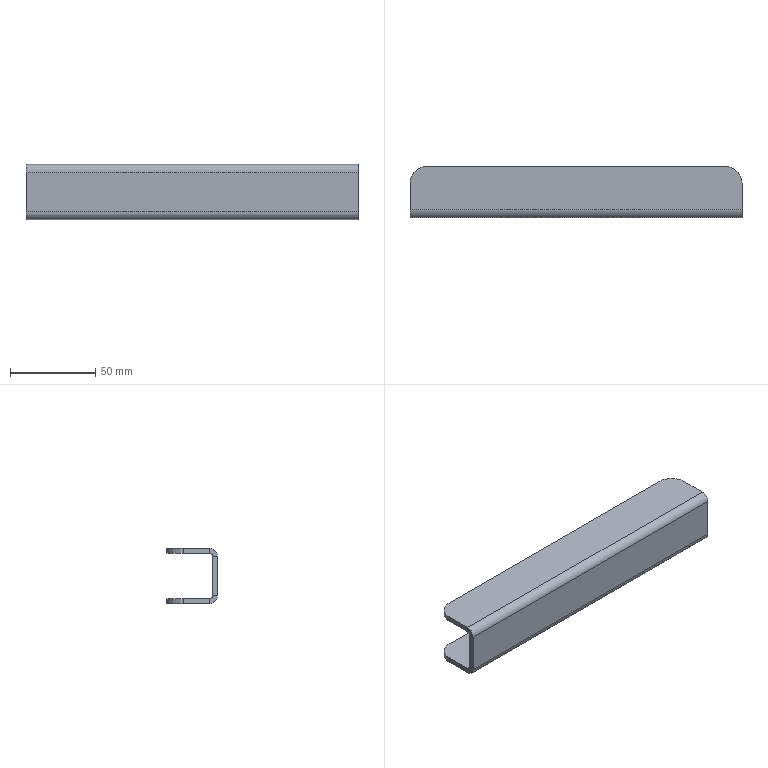Part | NX | features BREP 1 | 1 solid | 26 faces | box 195.072 x 29.972 x 32.487 mm | volume 48731 mm3 | plane 18 | cylinder 8 | commonest cylinder face diameters 19.964 x4 3.175 x2 9.169 x2
STEP:
#1=CARTESIAN_POINT('',(-97.536,0.,11.659));
#2=VERTEX_POINT('',#1);
#3=CARTESIAN_POINT('',(97.536,0.,11.659));
#4=VERTEX_POINT('',#3);
#5=CARTESIAN_POINT('',(-97.536,0.,11.659));
#6=DIRECTION('',(1.,0.,0.));
#7=VECTOR('',#6,1000.);
#8=LINE('',#5,#7);
#9=EDGE_CURVE('',#2,#4,#8,.T.);
#10=ORIENTED_EDGE('',*,*,#9,.T.);
#11=CARTESIAN_POINT('',(97.536,0.,-11.659));
#12=VERTEX_POINT('',#11);
#13=CARTESIAN_POINT('',(97.536,0.,11.659));
#14=DIRECTION('',(0.,0.,-1.));
#15=VECTOR('',#14,1000.);
#16=LINE('',#13,#15);
#17=EDGE_CURVE('',#4,#12,#16,.T.);
#18=ORIENTED_EDGE('',*,*,#17,.T.);
#19=CARTESIAN_POINT('',(-97.536,0.,-11.659));
#20=VERTEX_POINT('',#19);
#21=CARTESIAN_POINT('',(97.536,0.,-11.659));
#22=DIRECTION('',(-1.,0.,0.));
#23=VECTOR('',#22,1000.);
#24=LINE('',#21,#23);
#25=EDGE_CURVE('',#12,#20,#24,.T.);
#26=ORIENTED_EDGE('',*,*,#25,.T.);
#27=CARTESIAN_POINT('',(-97.536,0.,-11.659));
#28=DIRECTION('',(0.,0.,1.));
#29=VECTOR('',#28,1000.);
#30=LINE('',#27,#29);
#31=EDGE_CURVE('',#20,#2,#30,.T.);
#32=ORIENTED_EDGE('',*,*,#31,.T.);
#33=EDGE_LOOP('',(#10,#18,#26,#32));
#34=FACE_BOUND('',#33,.T.);
#35=CARTESIAN_POINT('',(0.,0.,0.));
#36=DIRECTION('',(0.,1.,0.));
#37=DIRECTION('',(1.,0.,0.));
#38=AXIS2_PLACEMENT_3D('',#35,#36,#37);
#39=PLANE('',#38);
#40=ADVANCED_FACE('',(#34),#39,.T.);
#41=CARTESIAN_POINT('',(-97.536,-2.997,-11.659));
#42=VERTEX_POINT('',#41);
#43=CARTESIAN_POINT('',(-97.536,0.,-11.659));
#44=DIRECTION('',(0.,-1.,0.));
#45=VECTOR('',#44,1000.);
#46=LINE('',#43,#45);
#47=EDGE_CURVE('',#20,#42,#46,.T.);
#48=ORIENTED_EDGE('',*,*,#47,.T.);
#49=CARTESIAN_POINT('',(-97.536,-2.997,11.659));
#50=VERTEX_POINT('',#49);
#51=CARTESIAN_POINT('',(-97.536,-2.997,-11.659));
#52=DIRECTION('',(0.,0.,1.));
#53=VECTOR('',#52,1000.);
#54=LINE('',#51,#53);
#55=EDGE_CURVE('',#42,#50,#54,.T.);
#56=ORIENTED_EDGE('',*,*,#55,.T.);
#57=CARTESIAN_POINT('',(-97.536,0.,11.659));
#58=DIRECTION('',(0.,-1.,0.));
#59=VECTOR('',#58,1000.);
#60=LINE('',#57,#59);
#61=EDGE_CURVE('',#2,#50,#60,.T.);
#62=ORIENTED_EDGE('',*,*,#61,.F.);
#63=ORIENTED_EDGE('',*,*,#31,.F.);
#64=EDGE_LOOP('',(#48,#56,#62,#63));
#65=FACE_BOUND('',#64,.T.);
#66=CARTESIAN_POINT('',(-97.536,-1.499,0.));
#67=DIRECTION('',(-1.,0.,0.));
#68=DIRECTION('',(0.,0.,1.));
#69=AXIS2_PLACEMENT_3D('',#66,#67,#68);
#70=PLANE('',#69);
#71=ADVANCED_FACE('',(#65),#70,.T.);
#72=ORIENTED_EDGE('',*,*,#61,.T.);
#73=CARTESIAN_POINT('',(-97.536,1.587,16.243));
#74=VERTEX_POINT('',#73);
#75=CARTESIAN_POINT('',(-97.536,1.587,11.659));
#76=DIRECTION('',(1.,0.,0.));
#77=DIRECTION('',(0.,0.,1.));
#78=AXIS2_PLACEMENT_3D('',#75,#76,#77);
#79=CIRCLE('',#78,4.585);
#80=EDGE_CURVE('',#74,#50,#79,.T.);
#81=ORIENTED_EDGE('',*,*,#80,.F.);
#82=CARTESIAN_POINT('',(-97.536,1.587,13.246));
#83=VERTEX_POINT('',#82);
#84=CARTESIAN_POINT('',(-97.536,1.587,13.246));
#85=DIRECTION('',(0.,0.,1.));
#86=VECTOR('',#85,1000.);
#87=LINE('',#84,#86);
#88=EDGE_CURVE('',#83,#74,#87,.T.);
#89=ORIENTED_EDGE('',*,*,#88,.F.);
#90=CARTESIAN_POINT('',(-97.536,1.587,11.659));
#91=DIRECTION('',(1.,0.,0.));
#92=DIRECTION('',(0.,0.,1.));
#93=AXIS2_PLACEMENT_3D('',#90,#91,#92);
#94=CIRCLE('',#93,1.587);
#95=EDGE_CURVE('',#83,#2,#94,.T.);
#96=ORIENTED_EDGE('',*,*,#95,.T.);
#97=EDGE_LOOP('',(#72,#81,#89,#96));
#98=FACE_BOUND('',#97,.T.);
#99=CARTESIAN_POINT('',(-97.536,-0.5947,13.841));
#100=DIRECTION('',(1.,0.,0.));
#101=DIRECTION('',(0.,1.,0.));
#102=AXIS2_PLACEMENT_3D('',#99,#100,#101);
#103=PLANE('',#102);
#104=ADVANCED_FACE('',(#98),#103,.F.);
#105=CARTESIAN_POINT('',(97.536,1.587,13.246));
#106=VERTEX_POINT('',#105);
#107=CARTESIAN_POINT('',(97.536,1.587,11.659));
#108=DIRECTION('',(1.,0.,0.));
#109=DIRECTION('',(0.,0.,1.));
#110=AXIS2_PLACEMENT_3D('',#107,#108,#109);
#111=CIRCLE('',#110,1.587);
#112=EDGE_CURVE('',#106,#4,#111,.T.);
#113=ORIENTED_EDGE('',*,*,#112,.T.);
#114=ORIENTED_EDGE('',*,*,#9,.F.);
#115=ORIENTED_EDGE('',*,*,#95,.F.);
#116=CARTESIAN_POINT('',(-97.536,1.587,13.246));
#117=DIRECTION('',(1.,0.,0.));
#118=VECTOR('',#117,1000.);
#119=LINE('',#116,#118);
#120=EDGE_CURVE('',#83,#106,#119,.T.);
#121=ORIENTED_EDGE('',*,*,#120,.T.);
#122=EDGE_LOOP('',(#113,#114,#115,#121));
#123=FACE_BOUND('',#122,.T.);
#124=CARTESIAN_POINT('',(-97.536,1.587,11.659));
#125=DIRECTION('',(1.,0.,0.));
#126=DIRECTION('',(0.,0.,1.));
#127=AXIS2_PLACEMENT_3D('',#124,#125,#126);
#128=CYLINDRICAL_SURFACE('',#127,1.587);
#129=ADVANCED_FACE('',(#123),#128,.F.);
#130=CARTESIAN_POINT('',(97.536,16.993,13.246));
#131=VERTEX_POINT('',#130);
#132=CARTESIAN_POINT('',(97.536,1.587,13.246));
#133=DIRECTION('',(0.,1.,0.));
#134=VECTOR('',#133,1000.);
#135=LINE('',#132,#134);
#136=EDGE_CURVE('',#106,#131,#135,.T.);
#137=ORIENTED_EDGE('',*,*,#136,.F.);
#138=ORIENTED_EDGE('',*,*,#120,.F.);
#139=CARTESIAN_POINT('',(-97.536,16.993,13.246));
#140=VERTEX_POINT('',#139);
#141=CARTESIAN_POINT('',(-97.536,16.993,13.246));
#142=DIRECTION('',(0.,-1.,0.));
#143=VECTOR('',#142,1000.);
#144=LINE('',#141,#143);
#145=EDGE_CURVE('',#140,#83,#144,.T.);
#146=ORIENTED_EDGE('',*,*,#145,.F.);
#147=CARTESIAN_POINT('',(-87.554,26.975,13.246));
#148=VERTEX_POINT('',#147);
#149=CARTESIAN_POINT('',(-87.554,16.993,13.246));
#150=DIRECTION('',(0.,0.,-1.));
#151=DIRECTION('',(-1.,0.,0.));
#152=AXIS2_PLACEMENT_3D('',#149,#150,#151);
#153=CIRCLE('',#152,9.982);
#154=EDGE_CURVE('',#140,#148,#153,.T.);
#155=ORIENTED_EDGE('',*,*,#154,.T.);
#156=CARTESIAN_POINT('',(87.554,26.975,13.246));
#157=VERTEX_POINT('',#156);
#158=CARTESIAN_POINT('',(87.554,26.975,13.246));
#159=DIRECTION('',(-1.,0.,0.));
#160=VECTOR('',#159,1000.);
#161=LINE('',#158,#160);
#162=EDGE_CURVE('',#157,#148,#161,.T.);
#163=ORIENTED_EDGE('',*,*,#162,.F.);
#164=CARTESIAN_POINT('',(87.554,16.993,13.246));
#165=DIRECTION('',(0.,0.,-1.));
#166=DIRECTION('',(0.,1.,0.));
#167=AXIS2_PLACEMENT_3D('',#164,#165,#166);
#168=CIRCLE('',#167,9.982);
#169=EDGE_CURVE('',#157,#131,#168,.T.);
#170=ORIENTED_EDGE('',*,*,#169,.T.);
#171=EDGE_LOOP('',(#137,#138,#146,#155,#163,#170));
#172=FACE_BOUND('',#171,.T.);
#173=CARTESIAN_POINT('',(-51.187,0.,13.246));
#174=DIRECTION('',(0.,0.,1.));
#175=DIRECTION('',(1.,0.,0.));
#176=AXIS2_PLACEMENT_3D('',#173,#174,#175);
#177=PLANE('',#176);
#178=ADVANCED_FACE('',(#172),#177,.F.);
#179=CARTESIAN_POINT('',(97.536,16.993,16.243));
#180=VERTEX_POINT('',#179);
#181=CARTESIAN_POINT('',(87.554,26.975,16.243));
#182=VERTEX_POINT('',#181);
#183=CARTESIAN_POINT('',(87.554,16.993,16.243));
#184=DIRECTION('',(0.,0.,1.));
#185=DIRECTION('',(1.,0.,0.));
#186=AXIS2_PLACEMENT_3D('',#183,#184,#185);
#187=CIRCLE('',#186,9.982);
#188=EDGE_CURVE('',#180,#182,#187,.T.);
#189=ORIENTED_EDGE('',*,*,#188,.F.);
#190=CARTESIAN_POINT('',(97.536,16.993,16.243));
#191=DIRECTION('',(0.,0.,-1.));
#192=VECTOR('',#191,1000.);
#193=LINE('',#190,#192);
#194=EDGE_CURVE('',#180,#131,#193,.T.);
#195=ORIENTED_EDGE('',*,*,#194,.T.);
#196=ORIENTED_EDGE('',*,*,#169,.F.);
#197=CARTESIAN_POINT('',(87.554,26.975,16.243));
#198=DIRECTION('',(0.,0.,-1.));
#199=VECTOR('',#198,1000.);
#200=LINE('',#197,#199);
#201=EDGE_CURVE('',#182,#157,#200,.T.);
#202=ORIENTED_EDGE('',*,*,#201,.F.);
#203=EDGE_LOOP('',(#189,#195,#196,#202));
#204=FACE_BOUND('',#203,.T.);
#205=CARTESIAN_POINT('',(87.554,16.993,16.533));
#206=DIRECTION('',(0.,0.,-1.));
#207=DIRECTION('',(0.,1.,0.));
#208=AXIS2_PLACEMENT_3D('',#205,#206,#207);
#209=CYLINDRICAL_SURFACE('',#208,9.982);
#210=ADVANCED_FACE('',(#204),#209,.T.);
#211=ORIENTED_EDGE('',*,*,#162,.T.);
#212=CARTESIAN_POINT('',(-87.554,26.975,16.243));
#213=VERTEX_POINT('',#212);
#214=CARTESIAN_POINT('',(-87.554,26.975,16.243));
#215=DIRECTION('',(0.,0.,-1.));
#216=VECTOR('',#215,1000.);
#217=LINE('',#214,#216);
#218=EDGE_CURVE('',#213,#148,#217,.T.);
#219=ORIENTED_EDGE('',*,*,#218,.F.);
#220=CARTESIAN_POINT('',(87.554,26.975,16.243));
#221=DIRECTION('',(-1.,0.,0.));
#222=VECTOR('',#221,1000.);
#223=LINE('',#220,#222);
#224=EDGE_CURVE('',#182,#213,#223,.T.);
#225=ORIENTED_EDGE('',*,*,#224,.F.);
#226=ORIENTED_EDGE('',*,*,#201,.T.);
#227=EDGE_LOOP('',(#211,#219,#225,#226));
#228=FACE_BOUND('',#227,.T.);
#229=CARTESIAN_POINT('',(0.,26.975,14.745));
#230=DIRECTION('',(0.,-1.,0.));
#231=DIRECTION('',(0.,0.,-1.));
#232=AXIS2_PLACEMENT_3D('',#229,#230,#231);
#233=PLANE('',#232);
#234=ADVANCED_FACE('',(#228),#233,.F.);
#235=ORIENTED_EDGE('',*,*,#224,.T.);
#236=CARTESIAN_POINT('',(-97.536,16.993,16.243));
#237=VERTEX_POINT('',#236);
#238=CARTESIAN_POINT('',(-87.554,16.993,16.243));
#239=DIRECTION('',(0.,0.,1.));
#240=DIRECTION('',(0.,1.,0.));
#241=AXIS2_PLACEMENT_3D('',#238,#239,#240);
#242=CIRCLE('',#241,9.982);
#243=EDGE_CURVE('',#213,#237,#242,.T.);
#244=ORIENTED_EDGE('',*,*,#243,.T.);
#245=CARTESIAN_POINT('',(-97.536,16.993,16.243));
#246=DIRECTION('',(0.,-1.,0.));
#247=VECTOR('',#246,1000.);
#248=LINE('',#245,#247);
#249=EDGE_CURVE('',#237,#74,#248,.T.);
#250=ORIENTED_EDGE('',*,*,#249,.T.);
#251=CARTESIAN_POINT('',(97.536,1.587,16.243));
#252=VERTEX_POINT('',#251);
#253=CARTESIAN_POINT('',(-97.536,1.587,16.243));
#254=DIRECTION('',(1.,0.,0.));
#255=VECTOR('',#254,1000.);
#256=LINE('',#253,#255);
#257=EDGE_CURVE('',#74,#252,#256,.T.);
#258=ORIENTED_EDGE('',*,*,#257,.T.);
#259=CARTESIAN_POINT('',(97.536,1.587,16.243));
#260=DIRECTION('',(0.,1.,0.));
#261=VECTOR('',#260,1000.);
#262=LINE('',#259,#261);
#263=EDGE_CURVE('',#252,#180,#262,.T.);
#264=ORIENTED_EDGE('',*,*,#263,.T.);
#265=ORIENTED_EDGE('',*,*,#188,.T.);
#266=EDGE_LOOP('',(#235,#244,#250,#258,#264,#265));
#267=FACE_BOUND('',#266,.T.);
#268=CARTESIAN_POINT('',(-51.187,0.,16.243));
#269=DIRECTION('',(0.,0.,1.));
#270=DIRECTION('',(1.,0.,0.));
#271=AXIS2_PLACEMENT_3D('',#268,#269,#270);
#272=PLANE('',#271);
#273=ADVANCED_FACE('',(#267),#272,.T.);
#274=ORIENTED_EDGE('',*,*,#263,.F.);
#275=CARTESIAN_POINT('',(97.536,1.587,13.246));
#276=DIRECTION('',(0.,0.,1.));
#277=VECTOR('',#276,1000.);
#278=LINE('',#275,#277);
#279=EDGE_CURVE('',#106,#252,#278,.T.);
#280=ORIENTED_EDGE('',*,*,#279,.F.);
#281=ORIENTED_EDGE('',*,*,#136,.T.);
#282=ORIENTED_EDGE('',*,*,#194,.F.);
#283=EDGE_LOOP('',(#274,#280,#281,#282));
#284=FACE_BOUND('',#283,.T.);
#285=CARTESIAN_POINT('',(97.536,14.281,14.745));
#286=DIRECTION('',(-1.,0.,0.));
#287=DIRECTION('',(0.,0.,1.));
#288=AXIS2_PLACEMENT_3D('',#285,#286,#287);
#289=PLANE('',#288);
#290=ADVANCED_FACE('',(#284),#289,.F.);
#291=ORIENTED_EDGE('',*,*,#279,.T.);
#292=CARTESIAN_POINT('',(97.536,-2.997,11.659));
#293=VERTEX_POINT('',#292);
#294=CARTESIAN_POINT('',(97.536,1.587,11.659));
#295=DIRECTION('',(1.,0.,0.));
#296=DIRECTION('',(0.,0.,1.));
#297=AXIS2_PLACEMENT_3D('',#294,#295,#296);
#298=CIRCLE('',#297,4.585);
#299=EDGE_CURVE('',#252,#293,#298,.T.);
#300=ORIENTED_EDGE('',*,*,#299,.T.);
#301=CARTESIAN_POINT('',(97.536,0.,11.659));
#302=DIRECTION('',(0.,-1.,0.));
#303=VECTOR('',#302,1000.);
#304=LINE('',#301,#303);
#305=EDGE_CURVE('',#4,#293,#304,.T.);
#306=ORIENTED_EDGE('',*,*,#305,.F.);
#307=ORIENTED_EDGE('',*,*,#112,.F.);
#308=EDGE_LOOP('',(#291,#300,#306,#307));
#309=FACE_BOUND('',#308,.T.);
#310=CARTESIAN_POINT('',(97.536,-0.5947,13.841));
#311=DIRECTION('',(1.,0.,0.));
#312=DIRECTION('',(0.,1.,0.));
#313=AXIS2_PLACEMENT_3D('',#310,#311,#312);
#314=PLANE('',#313);
#315=ADVANCED_FACE('',(#309),#314,.T.);
#316=ORIENTED_EDGE('',*,*,#305,.T.);
#317=CARTESIAN_POINT('',(97.536,-2.997,-11.659));
#318=VERTEX_POINT('',#317);
#319=CARTESIAN_POINT('',(97.536,-2.997,11.659));
#320=DIRECTION('',(0.,0.,-1.));
#321=VECTOR('',#320,1000.);
#322=LINE('',#319,#321);
#323=EDGE_CURVE('',#293,#318,#322,.T.);
#324=ORIENTED_EDGE('',*,*,#323,.T.);
#325=CARTESIAN_POINT('',(97.536,0.,-11.659));
#326=DIRECTION('',(0.,-1.,0.));
#327=VECTOR('',#326,1000.);
#328=LINE('',#325,#327);
#329=EDGE_CURVE('',#12,#318,#328,.T.);
#330=ORIENTED_EDGE('',*,*,#329,.F.);
#331=ORIENTED_EDGE('',*,*,#17,.F.);
#332=EDGE_LOOP('',(#316,#324,#330,#331));
#333=FACE_BOUND('',#332,.T.);
#334=CARTESIAN_POINT('',(97.536,-1.499,0.));
#335=DIRECTION('',(1.,0.,0.));
#336=DIRECTION('',(0.,1.,0.));
#337=AXIS2_PLACEMENT_3D('',#334,#335,#336);
#338=PLANE('',#337);
#339=ADVANCED_FACE('',(#333),#338,.T.);
#340=ORIENTED_EDGE('',*,*,#329,.T.);
#341=CARTESIAN_POINT('',(97.536,1.587,-16.243));
#342=VERTEX_POINT('',#341);
#343=CARTESIAN_POINT('',(97.536,1.587,-11.659));
#344=DIRECTION('',(-1.,0.,0.));
#345=DIRECTION('',(0.,0.,-1.));
#346=AXIS2_PLACEMENT_3D('',#343,#344,#345);
#347=CIRCLE('',#346,4.585);
#348=EDGE_CURVE('',#342,#318,#347,.T.);
#349=ORIENTED_EDGE('',*,*,#348,.F.);
#350=CARTESIAN_POINT('',(97.536,1.587,-13.246));
#351=VERTEX_POINT('',#350);
#352=CARTESIAN_POINT('',(97.536,1.587,-13.246));
#353=DIRECTION('',(0.,0.,-1.));
#354=VECTOR('',#353,1000.);
#355=LINE('',#352,#354);
#356=EDGE_CURVE('',#351,#342,#355,.T.);
#357=ORIENTED_EDGE('',*,*,#356,.F.);
#358=CARTESIAN_POINT('',(97.536,1.587,-11.659));
#359=DIRECTION('',(-1.,0.,0.));
#360=DIRECTION('',(0.,0.,-1.));
#361=AXIS2_PLACEMENT_3D('',#358,#359,#360);
#362=CIRCLE('',#361,1.587);
#363=EDGE_CURVE('',#351,#12,#362,.T.);
#364=ORIENTED_EDGE('',*,*,#363,.T.);
#365=EDGE_LOOP('',(#340,#349,#357,#364));
#366=FACE_BOUND('',#365,.T.);
#367=CARTESIAN_POINT('',(97.536,-0.5947,-13.841));
#368=DIRECTION('',(-1.,0.,0.));
#369=DIRECTION('',(0.,0.,1.));
#370=AXIS2_PLACEMENT_3D('',#367,#368,#369);
#371=PLANE('',#370);
#372=ADVANCED_FACE('',(#366),#371,.F.);
#373=CARTESIAN_POINT('',(-97.536,1.587,-13.246));
#374=VERTEX_POINT('',#373);
#375=CARTESIAN_POINT('',(-97.536,1.587,-11.659));
#376=DIRECTION('',(-1.,0.,0.));
#377=DIRECTION('',(0.,0.,-1.));
#378=AXIS2_PLACEMENT_3D('',#375,#376,#377);
#379=CIRCLE('',#378,1.587);
#380=EDGE_CURVE('',#374,#20,#379,.T.);
#381=ORIENTED_EDGE('',*,*,#380,.T.);
#382=ORIENTED_EDGE('',*,*,#25,.F.);
#383=ORIENTED_EDGE('',*,*,#363,.F.);
#384=CARTESIAN_POINT('',(97.536,1.587,-13.246));
#385=DIRECTION('',(-1.,0.,0.));
#386=VECTOR('',#385,1000.);
#387=LINE('',#384,#386);
#388=EDGE_CURVE('',#351,#374,#387,.T.);
#389=ORIENTED_EDGE('',*,*,#388,.T.);
#390=EDGE_LOOP('',(#381,#382,#383,#389));
#391=FACE_BOUND('',#390,.T.);
#392=CARTESIAN_POINT('',(97.536,1.587,-11.659));
#393=DIRECTION('',(-1.,0.,0.));
#394=DIRECTION('',(0.,0.,-1.));
#395=AXIS2_PLACEMENT_3D('',#392,#393,#394);
#396=CYLINDRICAL_SURFACE('',#395,1.587);
#397=ADVANCED_FACE('',(#391),#396,.F.);
#398=CARTESIAN_POINT('',(-87.554,26.975,-13.246));
#399=VERTEX_POINT('',#398);
#400=CARTESIAN_POINT('',(87.554,26.975,-13.246));
#401=VERTEX_POINT('',#400);
#402=CARTESIAN_POINT('',(-87.554,26.975,-13.246));
#403=DIRECTION('',(1.,0.,0.));
#404=VECTOR('',#403,1000.);
#405=LINE('',#402,#404);
#406=EDGE_CURVE('',#399,#401,#405,.T.);
#407=ORIENTED_EDGE('',*,*,#406,.F.);
#408=CARTESIAN_POINT('',(-97.536,16.993,-13.246));
#409=VERTEX_POINT('',#408);
#410=CARTESIAN_POINT('',(-87.554,16.993,-13.246));
#411=DIRECTION('',(0.,0.,1.));
#412=DIRECTION('',(0.,1.,0.));
#413=AXIS2_PLACEMENT_3D('',#410,#411,#412);
#414=CIRCLE('',#413,9.982);
#415=EDGE_CURVE('',#399,#409,#414,.T.);
#416=ORIENTED_EDGE('',*,*,#415,.T.);
#417=CARTESIAN_POINT('',(-97.536,1.587,-13.246));
#418=DIRECTION('',(0.,1.,0.));
#419=VECTOR('',#418,1000.);
#420=LINE('',#417,#419);
#421=EDGE_CURVE('',#374,#409,#420,.T.);
#422=ORIENTED_EDGE('',*,*,#421,.F.);
#423=ORIENTED_EDGE('',*,*,#388,.F.);
#424=CARTESIAN_POINT('',(97.536,16.993,-13.246));
#425=VERTEX_POINT('',#424);
#426=CARTESIAN_POINT('',(97.536,16.993,-13.246));
#427=DIRECTION('',(0.,-1.,0.));
#428=VECTOR('',#427,1000.);
#429=LINE('',#426,#428);
#430=EDGE_CURVE('',#425,#351,#429,.T.);
#431=ORIENTED_EDGE('',*,*,#430,.F.);
#432=CARTESIAN_POINT('',(87.554,16.993,-13.246));
#433=DIRECTION('',(0.,0.,1.));
#434=DIRECTION('',(1.,0.,0.));
#435=AXIS2_PLACEMENT_3D('',#432,#433,#434);
#436=CIRCLE('',#435,9.982);
#437=EDGE_CURVE('',#425,#401,#436,.T.);
#438=ORIENTED_EDGE('',*,*,#437,.T.);
#439=EDGE_LOOP('',(#407,#416,#422,#423,#431,#438));
#440=FACE_BOUND('',#439,.T.);
#441=CARTESIAN_POINT('',(51.187,0.,-13.246));
#442=DIRECTION('',(0.,0.,-1.));
#443=DIRECTION('',(0.,-1.,0.));
#444=AXIS2_PLACEMENT_3D('',#441,#442,#443);
#445=PLANE('',#444);
#446=ADVANCED_FACE('',(#440),#445,.F.);
#447=CARTESIAN_POINT('',(87.554,26.975,-16.243));
#448=VERTEX_POINT('',#447);
#449=CARTESIAN_POINT('',(97.536,16.993,-16.243));
#450=VERTEX_POINT('',#449);
#451=CARTESIAN_POINT('',(87.554,16.993,-16.243));
#452=DIRECTION('',(0.,0.,-1.));
#453=DIRECTION('',(0.,1.,0.));
#454=AXIS2_PLACEMENT_3D('',#451,#452,#453);
#455=CIRCLE('',#454,9.982);
#456=EDGE_CURVE('',#448,#450,#455,.T.);
#457=ORIENTED_EDGE('',*,*,#456,.F.);
#458=CARTESIAN_POINT('',(87.554,26.975,-16.243));
#459=DIRECTION('',(0.,0.,1.));
#460=VECTOR('',#459,1000.);
#461=LINE('',#458,#460);
#462=EDGE_CURVE('',#448,#401,#461,.T.);
#463=ORIENTED_EDGE('',*,*,#462,.T.);
#464=ORIENTED_EDGE('',*,*,#437,.F.);
#465=CARTESIAN_POINT('',(97.536,16.993,-16.243));
#466=DIRECTION('',(0.,0.,1.));
#467=VECTOR('',#466,1000.);
#468=LINE('',#465,#467);
#469=EDGE_CURVE('',#450,#425,#468,.T.);
#470=ORIENTED_EDGE('',*,*,#469,.F.);
#471=EDGE_LOOP('',(#457,#463,#464,#470));
#472=FACE_BOUND('',#471,.T.);
#473=CARTESIAN_POINT('',(87.554,16.993,-16.533));
#474=DIRECTION('',(0.,0.,1.));
#475=DIRECTION('',(1.,0.,0.));
#476=AXIS2_PLACEMENT_3D('',#473,#474,#475);
#477=CYLINDRICAL_SURFACE('',#476,9.982);
#478=ADVANCED_FACE('',(#472),#477,.T.);
#479=ORIENTED_EDGE('',*,*,#430,.T.);
#480=ORIENTED_EDGE('',*,*,#356,.T.);
#481=CARTESIAN_POINT('',(97.536,16.993,-16.243));
#482=DIRECTION('',(0.,-1.,0.));
#483=VECTOR('',#482,1000.);
#484=LINE('',#481,#483);
#485=EDGE_CURVE('',#450,#342,#484,.T.);
#486=ORIENTED_EDGE('',*,*,#485,.F.);
#487=ORIENTED_EDGE('',*,*,#469,.T.);
#488=EDGE_LOOP('',(#479,#480,#486,#487));
#489=FACE_BOUND('',#488,.T.);
#490=CARTESIAN_POINT('',(97.536,14.281,-14.745));
#491=DIRECTION('',(-1.,0.,0.));
#492=DIRECTION('',(0.,0.,1.));
#493=AXIS2_PLACEMENT_3D('',#490,#491,#492);
#494=PLANE('',#493);
#495=ADVANCED_FACE('',(#489),#494,.F.);
#496=ORIENTED_EDGE('',*,*,#485,.T.);
#497=CARTESIAN_POINT('',(-97.536,1.587,-16.243));
#498=VERTEX_POINT('',#497);
#499=CARTESIAN_POINT('',(97.536,1.587,-16.243));
#500=DIRECTION('',(-1.,0.,0.));
#501=VECTOR('',#500,1000.);
#502=LINE('',#499,#501);
#503=EDGE_CURVE('',#342,#498,#502,.T.);
#504=ORIENTED_EDGE('',*,*,#503,.T.);
#505=CARTESIAN_POINT('',(-97.536,16.993,-16.243));
#506=VERTEX_POINT('',#505);
#507=CARTESIAN_POINT('',(-97.536,1.587,-16.243));
#508=DIRECTION('',(0.,1.,0.));
#509=VECTOR('',#508,1000.);
#510=LINE('',#507,#509);
#511=EDGE_CURVE('',#498,#506,#510,.T.);
#512=ORIENTED_EDGE('',*,*,#511,.T.);
#513=CARTESIAN_POINT('',(-87.554,26.975,-16.243));
#514=VERTEX_POINT('',#513);
#515=CARTESIAN_POINT('',(-87.554,16.993,-16.243));
#516=DIRECTION('',(0.,0.,-1.));
#517=DIRECTION('',(-1.,0.,0.));
#518=AXIS2_PLACEMENT_3D('',#515,#516,#517);
#519=CIRCLE('',#518,9.982);
#520=EDGE_CURVE('',#506,#514,#519,.T.);
#521=ORIENTED_EDGE('',*,*,#520,.T.);
#522=CARTESIAN_POINT('',(-87.554,26.975,-16.243));
#523=DIRECTION('',(1.,0.,0.));
#524=VECTOR('',#523,1000.);
#525=LINE('',#522,#524);
#526=EDGE_CURVE('',#514,#448,#525,.T.);
#527=ORIENTED_EDGE('',*,*,#526,.T.);
#528=ORIENTED_EDGE('',*,*,#456,.T.);
#529=EDGE_LOOP('',(#496,#504,#512,#521,#527,#528));
#530=FACE_BOUND('',#529,.T.);
#531=CARTESIAN_POINT('',(51.187,0.,-16.243));
#532=DIRECTION('',(0.,0.,-1.));
#533=DIRECTION('',(0.,-1.,0.));
#534=AXIS2_PLACEMENT_3D('',#531,#532,#533);
#535=PLANE('',#534);
#536=ADVANCED_FACE('',(#530),#535,.T.);
#537=ORIENTED_EDGE('',*,*,#526,.F.);
#538=CARTESIAN_POINT('',(-87.554,26.975,-16.243));
#539=DIRECTION('',(0.,0.,1.));
#540=VECTOR('',#539,1000.);
#541=LINE('',#538,#540);
#542=EDGE_CURVE('',#514,#399,#541,.T.);
#543=ORIENTED_EDGE('',*,*,#542,.T.);
#544=ORIENTED_EDGE('',*,*,#406,.T.);
#545=ORIENTED_EDGE('',*,*,#462,.F.);
#546=EDGE_LOOP('',(#537,#543,#544,#545));
#547=FACE_BOUND('',#546,.T.);
#548=CARTESIAN_POINT('',(0.,26.975,-14.745));
#549=DIRECTION('',(0.,-1.,0.));
#550=DIRECTION('',(0.,0.,-1.));
#551=AXIS2_PLACEMENT_3D('',#548,#549,#550);
#552=PLANE('',#551);
#553=ADVANCED_FACE('',(#547),#552,.F.);
#554=ORIENTED_EDGE('',*,*,#520,.F.);
#555=CARTESIAN_POINT('',(-97.536,16.993,-16.243));
#556=DIRECTION('',(0.,0.,1.));
#557=VECTOR('',#556,1000.);
#558=LINE('',#555,#557);
#559=EDGE_CURVE('',#506,#409,#558,.T.);
#560=ORIENTED_EDGE('',*,*,#559,.T.);
#561=ORIENTED_EDGE('',*,*,#415,.F.);
#562=ORIENTED_EDGE('',*,*,#542,.F.);
#563=EDGE_LOOP('',(#554,#560,#561,#562));
#564=FACE_BOUND('',#563,.T.);
#565=CARTESIAN_POINT('',(-87.554,16.993,-16.533));
#566=DIRECTION('',(0.,0.,1.));
#567=DIRECTION('',(0.,1.,0.));
#568=AXIS2_PLACEMENT_3D('',#565,#566,#567);
#569=CYLINDRICAL_SURFACE('',#568,9.982);
#570=ADVANCED_FACE('',(#564),#569,.T.);
#571=ORIENTED_EDGE('',*,*,#511,.F.);
#572=CARTESIAN_POINT('',(-97.536,1.587,-13.246));
#573=DIRECTION('',(0.,0.,-1.));
#574=VECTOR('',#573,1000.);
#575=LINE('',#572,#574);
#576=EDGE_CURVE('',#374,#498,#575,.T.);
#577=ORIENTED_EDGE('',*,*,#576,.F.);
#578=ORIENTED_EDGE('',*,*,#421,.T.);
#579=ORIENTED_EDGE('',*,*,#559,.F.);
#580=EDGE_LOOP('',(#571,#577,#578,#579));
#581=FACE_BOUND('',#580,.T.);
#582=CARTESIAN_POINT('',(-97.536,14.281,-14.745));
#583=DIRECTION('',(1.,0.,0.));
#584=DIRECTION('',(0.,1.,0.));
#585=AXIS2_PLACEMENT_3D('',#582,#583,#584);
#586=PLANE('',#585);
#587=ADVANCED_FACE('',(#581),#586,.F.);
#588=ORIENTED_EDGE('',*,*,#576,.T.);
#589=CARTESIAN_POINT('',(-97.536,1.587,-11.659));
#590=DIRECTION('',(-1.,0.,0.));
#591=DIRECTION('',(0.,0.,-1.));
#592=AXIS2_PLACEMENT_3D('',#589,#590,#591);
#593=CIRCLE('',#592,4.585);
#594=EDGE_CURVE('',#498,#42,#593,.T.);
#595=ORIENTED_EDGE('',*,*,#594,.T.);
#596=ORIENTED_EDGE('',*,*,#47,.F.);
#597=ORIENTED_EDGE('',*,*,#380,.F.);
#598=EDGE_LOOP('',(#588,#595,#596,#597));
#599=FACE_BOUND('',#598,.T.);
#600=CARTESIAN_POINT('',(-97.536,-0.5947,-13.841));
#601=DIRECTION('',(-1.,0.,0.));
#602=DIRECTION('',(0.,0.,1.));
#603=AXIS2_PLACEMENT_3D('',#600,#601,#602);
#604=PLANE('',#603);
#605=ADVANCED_FACE('',(#599),#604,.T.);
#606=ORIENTED_EDGE('',*,*,#348,.T.);
#607=CARTESIAN_POINT('',(97.536,-2.997,-11.659));
#608=DIRECTION('',(-1.,0.,0.));
#609=VECTOR('',#608,1000.);
#610=LINE('',#607,#609);
#611=EDGE_CURVE('',#318,#42,#610,.T.);
#612=ORIENTED_EDGE('',*,*,#611,.T.);
#613=ORIENTED_EDGE('',*,*,#594,.F.);
#614=ORIENTED_EDGE('',*,*,#503,.F.);
#615=EDGE_LOOP('',(#606,#612,#613,#614));
#616=FACE_BOUND('',#615,.T.);
#617=CARTESIAN_POINT('',(97.536,1.587,-11.659));
#618=DIRECTION('',(-1.,0.,0.));
#619=DIRECTION('',(0.,0.,-1.));
#620=AXIS2_PLACEMENT_3D('',#617,#618,#619);
#621=CYLINDRICAL_SURFACE('',#620,4.585);
#622=ADVANCED_FACE('',(#616),#621,.T.);
#623=ORIENTED_EDGE('',*,*,#611,.F.);
#624=ORIENTED_EDGE('',*,*,#323,.F.);
#625=CARTESIAN_POINT('',(-97.536,-2.997,11.659));
#626=DIRECTION('',(1.,0.,0.));
#627=VECTOR('',#626,1000.);
#628=LINE('',#625,#627);
#629=EDGE_CURVE('',#50,#293,#628,.T.);
#630=ORIENTED_EDGE('',*,*,#629,.F.);
#631=ORIENTED_EDGE('',*,*,#55,.F.);
#632=EDGE_LOOP('',(#623,#624,#630,#631));
#633=FACE_BOUND('',#632,.T.);
#634=CARTESIAN_POINT('',(0.,-2.997,0.));
#635=DIRECTION('',(0.,1.,0.));
#636=DIRECTION('',(1.,0.,0.));
#637=AXIS2_PLACEMENT_3D('',#634,#635,#636);
#638=PLANE('',#637);
#639=ADVANCED_FACE('',(#633),#638,.F.);
#640=ORIENTED_EDGE('',*,*,#80,.T.);
#641=ORIENTED_EDGE('',*,*,#629,.T.);
#642=ORIENTED_EDGE('',*,*,#299,.F.);
#643=ORIENTED_EDGE('',*,*,#257,.F.);
#644=EDGE_LOOP('',(#640,#641,#642,#643));
#645=FACE_BOUND('',#644,.T.);
#646=CARTESIAN_POINT('',(-97.536,1.587,11.659));
#647=DIRECTION('',(1.,0.,0.));
#648=DIRECTION('',(0.,0.,1.));
#649=AXIS2_PLACEMENT_3D('',#646,#647,#648);
#650=CYLINDRICAL_SURFACE('',#649,4.585);
#651=ADVANCED_FACE('',(#645),#650,.T.);
#652=ORIENTED_EDGE('',*,*,#145,.T.);
#653=ORIENTED_EDGE('',*,*,#88,.T.);
#654=ORIENTED_EDGE('',*,*,#249,.F.);
#655=CARTESIAN_POINT('',(-97.536,16.993,16.243));
#656=DIRECTION('',(0.,0.,-1.));
#657=VECTOR('',#656,1000.);
#658=LINE('',#655,#657);
#659=EDGE_CURVE('',#237,#140,#658,.T.);
#660=ORIENTED_EDGE('',*,*,#659,.T.);
#661=EDGE_LOOP('',(#652,#653,#654,#660));
#662=FACE_BOUND('',#661,.T.);
#663=CARTESIAN_POINT('',(-97.536,14.281,14.745));
#664=DIRECTION('',(1.,0.,0.));
#665=DIRECTION('',(0.,1.,0.));
#666=AXIS2_PLACEMENT_3D('',#663,#664,#665);
#667=PLANE('',#666);
#668=ADVANCED_FACE('',(#662),#667,.F.);
#669=ORIENTED_EDGE('',*,*,#243,.F.);
#670=ORIENTED_EDGE('',*,*,#218,.T.);
#671=ORIENTED_EDGE('',*,*,#154,.F.);
#672=ORIENTED_EDGE('',*,*,#659,.F.);
#673=EDGE_LOOP('',(#669,#670,#671,#672));
#674=FACE_BOUND('',#673,.T.);
#675=CARTESIAN_POINT('',(-87.554,16.993,16.533));
#676=DIRECTION('',(0.,0.,-1.));
#677=DIRECTION('',(-1.,0.,0.));
#678=AXIS2_PLACEMENT_3D('',#675,#676,#677);
#679=CYLINDRICAL_SURFACE('',#678,9.982);
#680=ADVANCED_FACE('',(#674),#679,.T.);
#681=CLOSED_SHELL('',(#40,#71,#104,#129,#178,#210,#234,#273,#290,#315,#339,#372,#397,#446,#478,#495,#536,#553,#570,#587,#605,#622,#639,#651,#668,#680));
#682=MANIFOLD_SOLID_BREP('',#681);
#683=(LENGTH_UNIT()NAMED_UNIT(*)SI_UNIT(.MILLI.,.METRE.));
#684=UNCERTAINTY_MEASURE_WITH_UNIT(LENGTH_MEASURE(0.00001),#683,'','');
#685=(NAMED_UNIT(*)PLANE_ANGLE_UNIT()SI_UNIT($,.RADIAN.));
#686=(NAMED_UNIT(*)SI_UNIT($,.STERADIAN.)SOLID_ANGLE_UNIT());
#687=(GEOMETRIC_REPRESENTATION_CONTEXT(3)GLOBAL_UNCERTAINTY_ASSIGNED_CONTEXT((#684))GLOBAL_UNIT_ASSIGNED_CONTEXT((#683,#685,#686))REPRESENTATION_CONTEXT('',''));
#688=ADVANCED_BREP_SHAPE_REPRESENTATION('',(#682),#687);